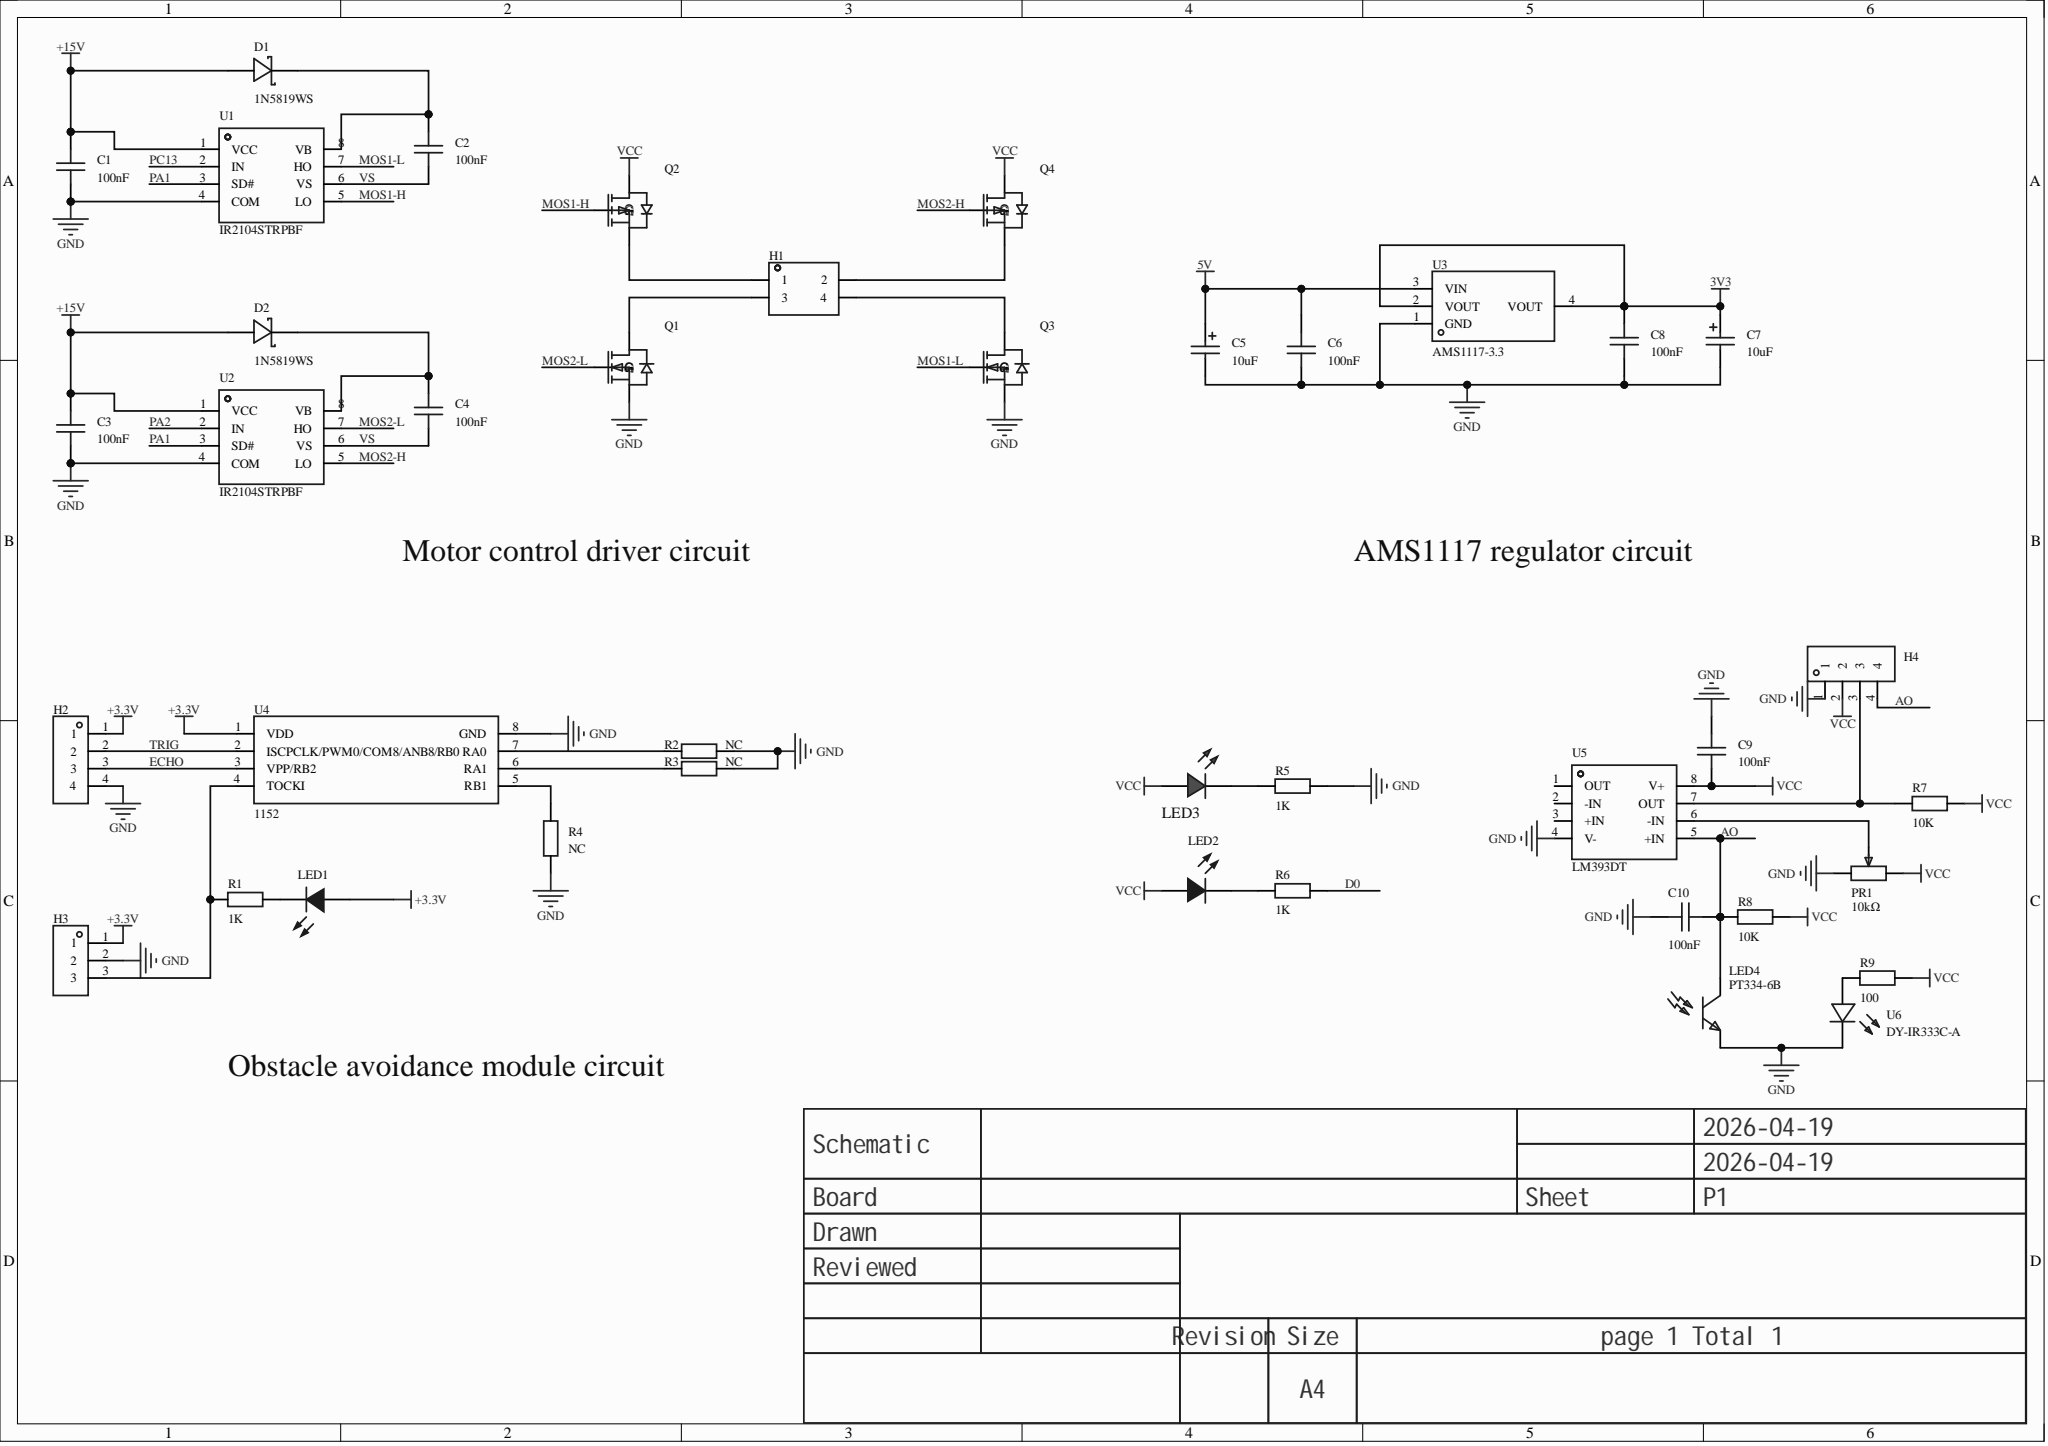Circuit board | Altium Designer | 40 parts | 31 nets
Bill of materials:
Comment,Description,Designator,Footprint,LibRef,Quantity
"100nF","","C1, C2, C3, C4, C6, C8, C9, C10","C0603","CAP_0603","8"
"10uF","","C5, C7","C_Ele_SMD_3x5.4mm","C_Ele_SMD_3x5.4mm","2"
"1N5819WS","Forward voltage drop (Vf): 600mV@1A; DC reverse voltage (Vr): 40V; rectified current: 1A;","D1, D2","SOD-323_L1.8-W1.3-LS2.5-RD","1N5819WS_C191023","2"
"","","H1","HDR-TH_4P-P2.54-V-F-R2-C2-S2.54","HDR-F_2.54_2x2","1"
"","","H2","HDR-TH_4P-P2.54-V-F","HDR-F_2.54_1x4P","1"
"","","H3","HDR-TH_3P-P2.54-V-F","HDR-F_2.54_1x3P","1"
"","","H4","HDR-TH_4P-P2.54-V-M","HDR-M_2.54_1x4P","1"
"","","LED1, LED2, LED3","LED_0603","LED_0603-B, LED_0603-R","3"
"PT334-6B","Transistor type: NPN; collector-emitter breakdown voltage (Vceo): 30V; collector current (Ic): 20mA; power dissipation (Pd): 75mW; dark current: 100nA; peak wavelength: 940nm;","LED4","LED-TH_BD5.9-P2.54-FD","PT334-6B","1"
"10kΩ","","PR1","R_3296","R_3296","1"
"","","Q1, Q3","SOT-23-3_L2.9-W1.3-P1.90-LS2.4-BR","AO3400A_N","2"
"","","Q2, Q4","AO3401A_SOT-23-3","AO3401A_P","2"
"1K","","R1, R5, R6","R0603","Res_0603","3"
"NC","","R2, R3, R4","R0603","Res_0603","3"
"10K","","R7, R8","R0603","Res_0603","2"
"100","","R9","R0603","Res_0603","1"
"IR2104STRPBF","Driver configuration: half-bridge; load type: IGBT; MOSFET; driver channels: 2; sink current (IOL): 270mA; source current (IOH): 130mA; operating voltage: 10V~20V; rise time (tr): 100ns; fall time (tf): 50ns;","U1, U2","SOIC-8_L4.9-W3.9-P1.27-LS6.0-BL","IR2104STRPBF","2"
"AMS1117-3.3","Output type: fixed; operating voltage: 15V; output voltage: 3.3V; output current: 1A; power supply ripple rejection (PSRR): 72dB@(120Hz); output polarity: positive;","U3","SOT-223-3_L6.5-W3.4-P2.30-LS7.0-BR","AMS1117-3.3_C6186","1"
"1152","","U4","SOP-8_L4.9-W3.9-P1.27-LS6.0-BL","KS2505SOP8_SOP8","1"
"LM393DT","Comparator count: dual; input offset voltage (Vos): 1mV; input bias current (Ib): 20nA;","U5","SOIC-8_L5.0-W4.0-P1.27-LS6.0-BL","LM393DT","1"
"DY-IR333C-A","Forward voltage drop (Vf): 1.2V~1.85V; power dissipation (Pd): 150mW; wavelength: 940nm; radiant intensity: 85mW/sr; forward current: 25mA; DC reverse voltage (Vr): 5V; viewing angle: 20°;","U6","LED-TH_BD5.9-P2.54-FD","DY-IR333C-A_C390046","1"
Netlist (Protel format):
[
C1
C0603
100nF



]
[
C2
C0603
100nF



]
[
C3
C0603
100nF



]
[
C4
C0603
100nF



]
[
C5
C_Ele_SMD_3x5.4mm
10uF



]
[
C6
C0603
100nF



]
[
C7
C_Ele_SMD_3x5.4mm
10uF



]
[
C8
C0603
100nF



]
[
C9
C0603
100nF



]
[
C10
C0603
100nF



]
[
D1
SOD-323_L1.8-W1.3-LS2.5-RD
1N5819WS



]
[
D2
SOD-323_L1.8-W1.3-LS2.5-RD
1N5819WS



]
[
H1
HDR-TH_4P-P2.54-V-F-R2-C2-S2.54




]
[
H2
HDR-TH_4P-P2.54-V-F




]
[
H3
HDR-TH_3P-P2.54-V-F




]
[
H4
HDR-TH_4P-P2.54-V-M




]
[
LED1
LED_0603




]
[
LED2
LED_0603




]
[
LED3
LED_0603




]
[
LED4
LED-TH_BD5.9-P2.54-FD
PT334-6B



]
[
PR1
R_3296
10kΩ



]
[
Q1
SOT-23-3_L2.9-W1.3-P1.90-LS2.4-BR




]
[
Q2
AO3401A_SOT-23-3




]
[
Q3
SOT-23-3_L2.9-W1.3-P1.90-LS2.4-BR




]
[
Q4
AO3401A_SOT-23-3




]
[
R1
R0603
1K



]
[
R2
R0603
NC



]
[
R3
R0603
NC



]
[
R4
R0603
NC



]
[
R5
R0603
1K



]
[
R6
R0603
1K



]
[
R7
R0603
10K



]
[
R8
R0603
10K



]
[
R9
R0603
100



]
[
U1
SOIC-8_L4.9-W3.9-P1.27-LS6.0-BL
IR2104STRPBF



]
[
U2
SOIC-8_L4.9-W3.9-P1.27-LS6.0-BL
IR2104STRPBF



]
[
U3
SOT-223-3_L6.5-W3.4-P2.30-LS7.0-BR
AMS1117-3.3



]
[
U4
SOP-8_L4.9-W3.9-P1.27-LS6.0-BL
1152



]
[
U5
SOIC-8_L5.0-W4.0-P1.27-LS6.0-BL
LM393DT



]
[
U6
LED-TH_BD5.9-P2.54-FD
DY-IR333C-A



]
(
VS
C2-1
C4-1
U1-6
U2-6
)
(
VCC
C9-1
H4-2
LED2-2
LED3-2
PR1-1
Q2-3
Q4-3
R7-2
R8-2
R9-2
U5-8
)
(
TRIG
H2-2
U4-2
)
(
PA1
U1-3
U2-3
)
(
NetR9_1
R9-1
U6-1
)
(
NetR4_1
R4-1
U4-5
)
(
NetR3_1
R3-1
U4-6
)
(
NetR2_1
R2-1
U4-7
)
(
NetPR1_2
PR1-2
U5-6
)
(
NetLED3_1
LED3-1
R5-1
)
(
NetLED2_1
LED2-1
R6-1
)
(
NetLED1_1
LED1-1
R1-2
)
(
NetH4_3
H4-3
R7-1
U5-7
)
(
NetH3_3
H3-3
R1-1
U4-4
)
(
NetH1_4
H1-4
Q3-3
)
(
NetH1_3
H1-3
Q1-3
)
(
NetH1_2
H1-2
Q4-2
)
(
NetH1_1
H1-1
Q2-2
)
(
NetC4_2
C4-2
D2-1
U2-8
)
(
NetC2_2
C2-2
D1-1
U1-8
)
(
MOS2-L
Q1-1
U2-7
)
(
MOS2-H
Q4-1
U2-5
)
(
MOS1-L
Q3-1
U1-7
)
(
MOS1-H
Q2-1
U1-5
)
(
GND
C1-1
C3-1
C5-2
C6-1
C7-2
C8-1
C9-2
C10-1
H2-4
H3-2
H4-1
LED4-1
PR1-3
Q1-2
Q3-2
R2-2
R3-2
R4-2
R5-2
U1-4
U2-4
U3-1
U4-8
U5-4
U6-2
)
(
ECHO
H2-3
U4-3
)
(
AO
C10-2
H4-4
LED4-2
R8-1
U5-5
)
(
+15V
C1-2
C3-2
D1-2
D2-2
U1-1
U2-1
)
(
+3.3V
H2-1
H3-1
LED1-2
U4-1
)
(
5V
C5-1
C6-2
U3-3
)
(
3V3
C7-1
C8-2
U3-2
U3-4
)